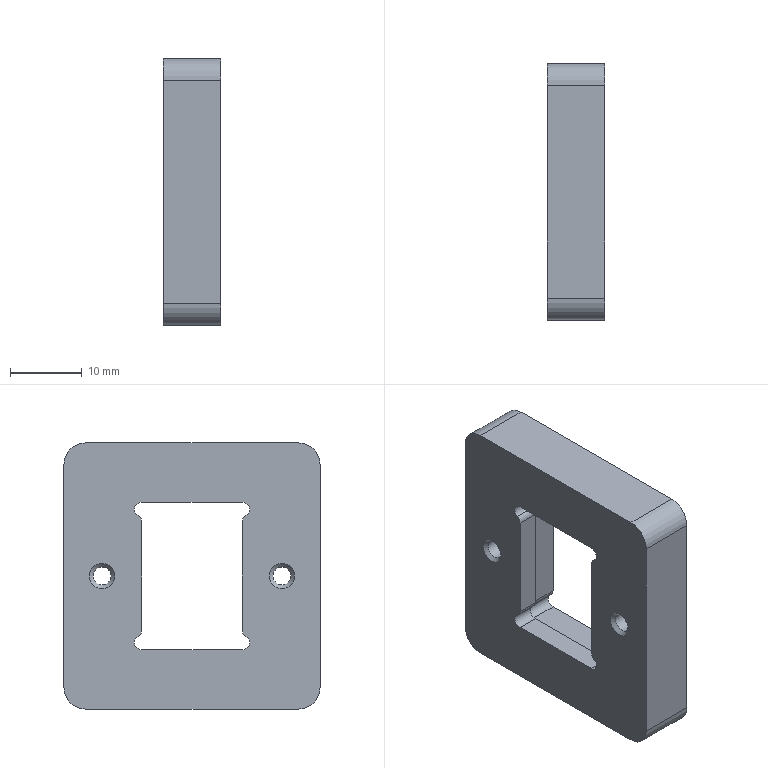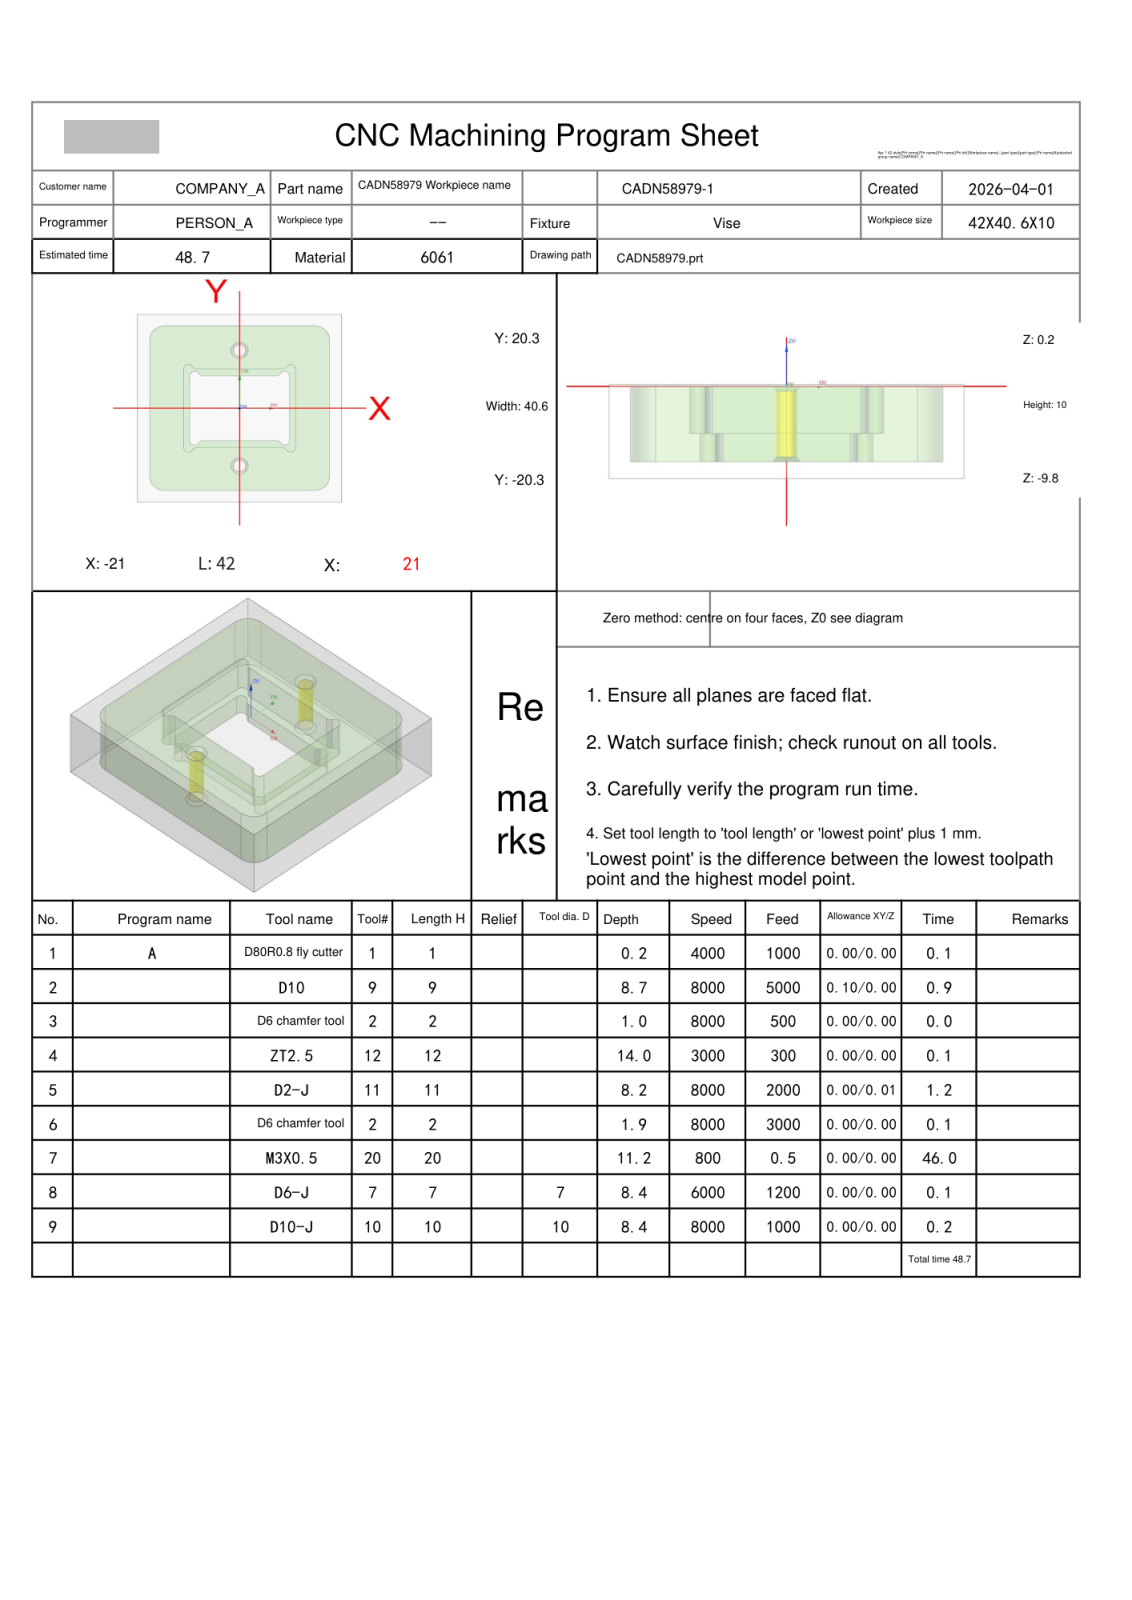NC program | NX | posted by the shop | part box 8 x 35.6 x 37 mm
Lines 1 to 314 of 3954:
%
O0001
(Machine time: 92.66 MIN)
(===Total Tool:8===)
(T1=D80R0.8 fly cutter D=80.  R=0.8  D-  H01 Z=-0.   )
(T9=D10     D=10.  R=0.   D-  H09 Z=-8.5  )
(T2=D6 chamfer tool   D=6.   R=0.   D-  H02 Z=-1.75 )
(T12=ZT2.5  D=2.5  DR_a=118 D-  H12 Z=-13.75)
(T11=D2-J   D=2.   R=0.   D-  H11 Z=-8.   )
(T20=M3X0.5 D=2.5  DR_a=180 D-  H20 Z=-11.  )
(T7=D6-J    D=6.   R=0.   D7  H07 Z=-8.2  )
(T10=D10-J  D=10.  R=0.   D10 H10 Z=-8.2  )
G80 G90 G17 G49 G40
G91 G28 Z0
M01
N1 T01 M06
(D80R0.8 fly cutter  D=80. R=0.8 H=01 ce=0.00 di=0.00)
G00 G90 G54 X-63.5 Y0.0 M03 S4000
G43 H01 Z20.
M08
Z2.
G01 Z0.0 F1000.
X-58.5
X58.5
X63.5
Z2.
G00 Z20.
G91 G28 Z0.0
M05
M09
G91 G28 Z0.0
M01
N2 T09 M06
(D10  D=10. R=0. H=09 ce=0.10 di=0.00)
G00 G90 G54 X0.0 Y22.9 M03 S8000
G43 H09 Z20.
M08
Z.5
G01 X15.5 Z.43 F5000.
G02 X23.6 Y14.8 Z.372 I0.0 J-8.1
G01 Y-14.8 Z.237
G02 X15.5 Y-22.9 Z.18 I-8.1 J0.0
G01 X-15.5 Z.039
G02 X-23.6 Y-14.8 Z-.019 I0.0 J8.1
G01 Y14.8 Z-.154
G02 X-15.5 Y22.9 Z-.211 I8.1 J0.0
G01 X15.5 Z-.352
G02 X23.6 Y14.8 Z-.41 I0.0 J-8.1
G01 Y-14.8 Z-.545
G02 X15.5 Y-22.9 Z-.602 I-8.1 J0.0
G01 X-15.5 Z-.743
G02 X-23.6 Y-14.8 Z-.801 I0.0 J8.1
G01 Y14.8 Z-.935
G02 X-15.5 Y22.9 Z-.993 I8.1 J0.0
G01 X15.5 Z-1.134
G02 X23.6 Y14.8 Z-1.192 I0.0 J-8.1
G01 Y-14.8 Z-1.326
G02 X15.5 Y-22.9 Z-1.384 I-8.1 J0.0
G01 X-15.5 Z-1.525
G02 X-23.6 Y-14.8 Z-1.583 I0.0 J8.1
G01 Y14.8 Z-1.717
G02 X-15.5 Y22.9 Z-1.775 I8.1 J0.0
G01 X15.5 Z-1.916
G02 X23.6 Y14.8 Z-1.974 I0.0 J-8.1
G01 Y-14.8 Z-2.108
G02 X15.5 Y-22.9 Z-2.166 I-8.1 J0.0
G01 X-15.5 Z-2.307
G02 X-23.6 Y-14.8 Z-2.365 I0.0 J8.1
G01 Y14.8 Z-2.499
G02 X-15.5 Y22.9 Z-2.557 I8.1 J0.0
G01 X15.5 Z-2.698
G02 X23.6 Y14.8 Z-2.755 I0.0 J-8.1
G01 Y-14.8 Z-2.89
G02 X15.5 Y-22.9 Z-2.948 I-8.1 J0.0
G01 X-15.5 Z-3.089
G02 X-23.6 Y-14.8 Z-3.146 I0.0 J8.1
G01 Y14.8 Z-3.281
G02 X-15.5 Y22.9 Z-3.339 I8.1 J0.0
G01 X15.5 Z-3.48
G02 X23.6 Y14.8 Z-3.537 I0.0 J-8.1
G01 Y-14.8 Z-3.672
G02 X15.5 Y-22.9 Z-3.73 I-8.1 J0.0
G01 X-15.5 Z-3.87
G02 X-23.6 Y-14.8 Z-3.928 I0.0 J8.1
G01 Y14.8 Z-4.063
G02 X-15.5 Y22.9 Z-4.12 I8.1 J0.0
G01 X15.5 Z-4.261
G02 X23.6 Y14.8 Z-4.319 I0.0 J-8.1
G01 Y-14.8 Z-4.454
G02 X15.5 Y-22.9 Z-4.511 I-8.1 J0.0
G01 X-15.5 Z-4.652
G02 X-23.6 Y-14.8 Z-4.71 I0.0 J8.1
G01 Y14.8 Z-4.845
G02 X-15.5 Y22.9 Z-4.902 I8.1 J0.0
G01 X15.5 Z-5.043
G02 X23.6 Y14.8 Z-5.101 I0.0 J-8.1
G01 Y-14.8 Z-5.235
G02 X15.5 Y-22.9 Z-5.293 I-8.1 J0.0
G01 X-15.5 Z-5.434
G02 X-23.6 Y-14.8 Z-5.492 I0.0 J8.1
G01 Y14.8 Z-5.626
G02 X-15.5 Y22.9 Z-5.684 I8.1 J0.0
G01 X15.5 Z-5.825
G02 X23.6 Y14.8 Z-5.883 I0.0 J-8.1
G01 Y-14.8 Z-6.017
G02 X15.5 Y-22.9 Z-6.075 I-8.1 J0.0
G01 X-15.5 Z-6.216
G02 X-23.6 Y-14.8 Z-6.274 I0.0 J8.1
G01 Y14.8 Z-6.408
G02 X-15.5 Y22.9 Z-6.466 I8.1 J0.0
G01 X15.5 Z-6.607
G02 X23.6 Y14.8 Z-6.665 I0.0 J-8.1
G01 Y-14.8 Z-6.799
G02 X15.5 Y-22.9 Z-6.857 I-8.1 J0.0
G01 X-15.5 Z-6.998
G02 X-23.6 Y-14.8 Z-7.055 I0.0 J8.1
G01 Y14.8 Z-7.19
G02 X-15.5 Y22.9 Z-7.248 I8.1 J0.0
G01 X15.5 Z-7.389
G02 X23.6 Y14.8 Z-7.446 I0.0 J-8.1
G01 Y-14.8 Z-7.581
G02 X15.5 Y-22.9 Z-7.639 I-8.1 J0.0
G01 X-15.5 Z-7.78
G02 X-23.6 Y-14.8 Z-7.837 I0.0 J8.1
G01 Y14.8 Z-7.972
G02 X-15.5 Y22.9 Z-8.03 I8.1 J0.0
G01 X0.0 Z-8.1
X15.5
G02 X23.6 Y14.8 I0.0 J-8.1
G01 Y-14.8
G02 X15.5 Y-22.9 I-8.1 J0.0
G01 X-15.5
G02 X-23.6 Y-14.8 I0.0 J8.1
G01 Y14.8
G02 X-15.5 Y22.9 I8.1 J0.0
G01 X0.0
X.5
Z-7.1
G00 Z20.
G00 G90 X-5.881 Y-3.4 M03 S8000
Z20.
Z1.
G01 X6.4 Z.356 F2000.
Y3.4 Z0.0
X-6.4 Z-.107
Y-3.4 Z-.163
X6.4 Z-.27
Y3.4 Z-.327
X-6.4 Z-.433
Y-3.4 Z-.49
X6.4 Z-.597
Y3.4 Z-.653
X-6.4 Z-.76
Y-3.4 Z-.817
X6.4 Z-.923
Y3.4 Z-.98
X-6.4 Z-1.087
Y-3.4 Z-1.143
X6.4 Z-1.25
Y3.4 Z-1.307
X-6.4 Z-1.413
Y-3.4 Z-1.47
X6.4 Z-1.577
Y3.4 Z-1.633
X-6.4 Z-1.74
Y-3.4 Z-1.797
X6.4 Z-1.903
Y3.4 Z-1.96
X-6.4 Z-2.067
Y-3.4 Z-2.123
X6.4 Z-2.23
Y3.4 Z-2.287
X-6.4 Z-2.393
Y-3.4 Z-2.45
X6.4 Z-2.557
Y3.4 Z-2.613
X-6.4 Z-2.72
Y-3.4 Z-2.777
X6.4 Z-2.883
Y3.4 Z-2.94
X-6.4 Z-3.047
Y-3.4 Z-3.103
X6.4 Z-3.21
Y3.4 Z-3.267
X-6.4 Z-3.373
Y-3.4 Z-3.43
X6.4 Z-3.537
Y3.4 Z-3.593
X-6.4 Z-3.7
Y-3.4 Z-3.757
X6.4 Z-3.863
Y3.4 Z-3.92
X-6.4 Z-4.027
Y-3.4 Z-4.083
X6.4 Z-4.19
Y3.4 Z-4.247
X-6.4 Z-4.353
Y-3.4 Z-4.41
X6.4 Z-4.517
Y3.4 Z-4.573
X-6.4 Z-4.68
Y-3.4 Z-4.737
X6.4 Z-4.843
Y3.4 Z-4.9
X-6.4
Y-3.4
X6.4
Y3.4
X6.
Z-3.9
G00 Z20.
G00 G90 X0.0 Y-1.9 M03 S6000
Z20.
Z-4.5
G01 X5.15 Z-4.552 F2500.
Y1.9 Z-4.591
X-5.15 Z-4.695
Y-1.9 Z-4.734
X5.15 Z-4.838
Y1.9 Z-4.876
X-5.15 Z-4.981
Y-1.9 Z-5.019
X5.15 Z-5.124
Y1.9 Z-5.162
X-5.15 Z-5.266
Y-1.9 Z-5.305
X5.15 Z-5.409
Y1.9 Z-5.448
X-5.15 Z-5.552
Y-1.9 Z-5.591
X5.15 Z-5.695
Y1.9 Z-5.734
X-5.15 Z-5.838
Y-1.9 Z-5.876
X5.15 Z-5.981
Y1.9 Z-6.019
X-5.15 Z-6.124
Y-1.9 Z-6.162
X5.15 Z-6.266
Y1.9 Z-6.305
X-5.15 Z-6.409
Y-1.9 Z-6.448
X5.15 Z-6.552
Y1.9 Z-6.591
X-5.15 Z-6.695
Y-1.9 Z-6.734
X5.15 Z-6.838
Y1.9 Z-6.876
X-5.15 Z-6.981
Y-1.9 Z-7.019
X5.15 Z-7.124
Y1.9 Z-7.162
X-5.15 Z-7.266
Y-1.9 Z-7.305
X5.15 Z-7.409
Y1.9 Z-7.448
X-5.15 Z-7.552
Y-1.9 Z-7.591
X5.15 Z-7.695
Y1.9 Z-7.734
X-5.15 Z-7.838
Y-1.9 Z-7.876
X5.15 Z-7.981
Y1.9 Z-8.019
X-5.15 Z-8.124
Y-1.9 Z-8.162
X5.15 Z-8.266
Y1.9 Z-8.305
X-5.15 Z-8.409
Y-1.9 Z-8.448
X0.0 Z-8.5
X5.15
Y1.9
X-5.15
Y-1.9
X0.0
X.5
Z-7.5
G00 Z20.
G91 G28 Z0.0
M05
M09
G91 G28 Z0.0
M01
N3 T02 M06
(D6 chamfer tool  D=6. R=0. H=02 ce=0.00 di=0.10)
G00 G90 G54 X0.0 Y-12.5 M03 S8000
G43 H02 Z20.
M08
G98 G81 X0.0 Y-12.5 Z-.8 R1. F500.
Y12.5
G80
G00 Z20.
G91 G28 Z0.0
M05
M09
G91 G28 Z0.0
M01
N4 T12 M06
(ZT2.5 D=2.5 DR_a=118 H=12)
G00 G90 G54 X0.0 Y-12.5 M03 S3000
G43 H12 Z20.
M08
G98 G83 X0.0 Y-12.5 Z-13.751 R1. F300. Q2.
Y12.5
G80
G00 Z20.
G91 G28 Z0.0
M05
M09
G91 G28 Z0.0
M01